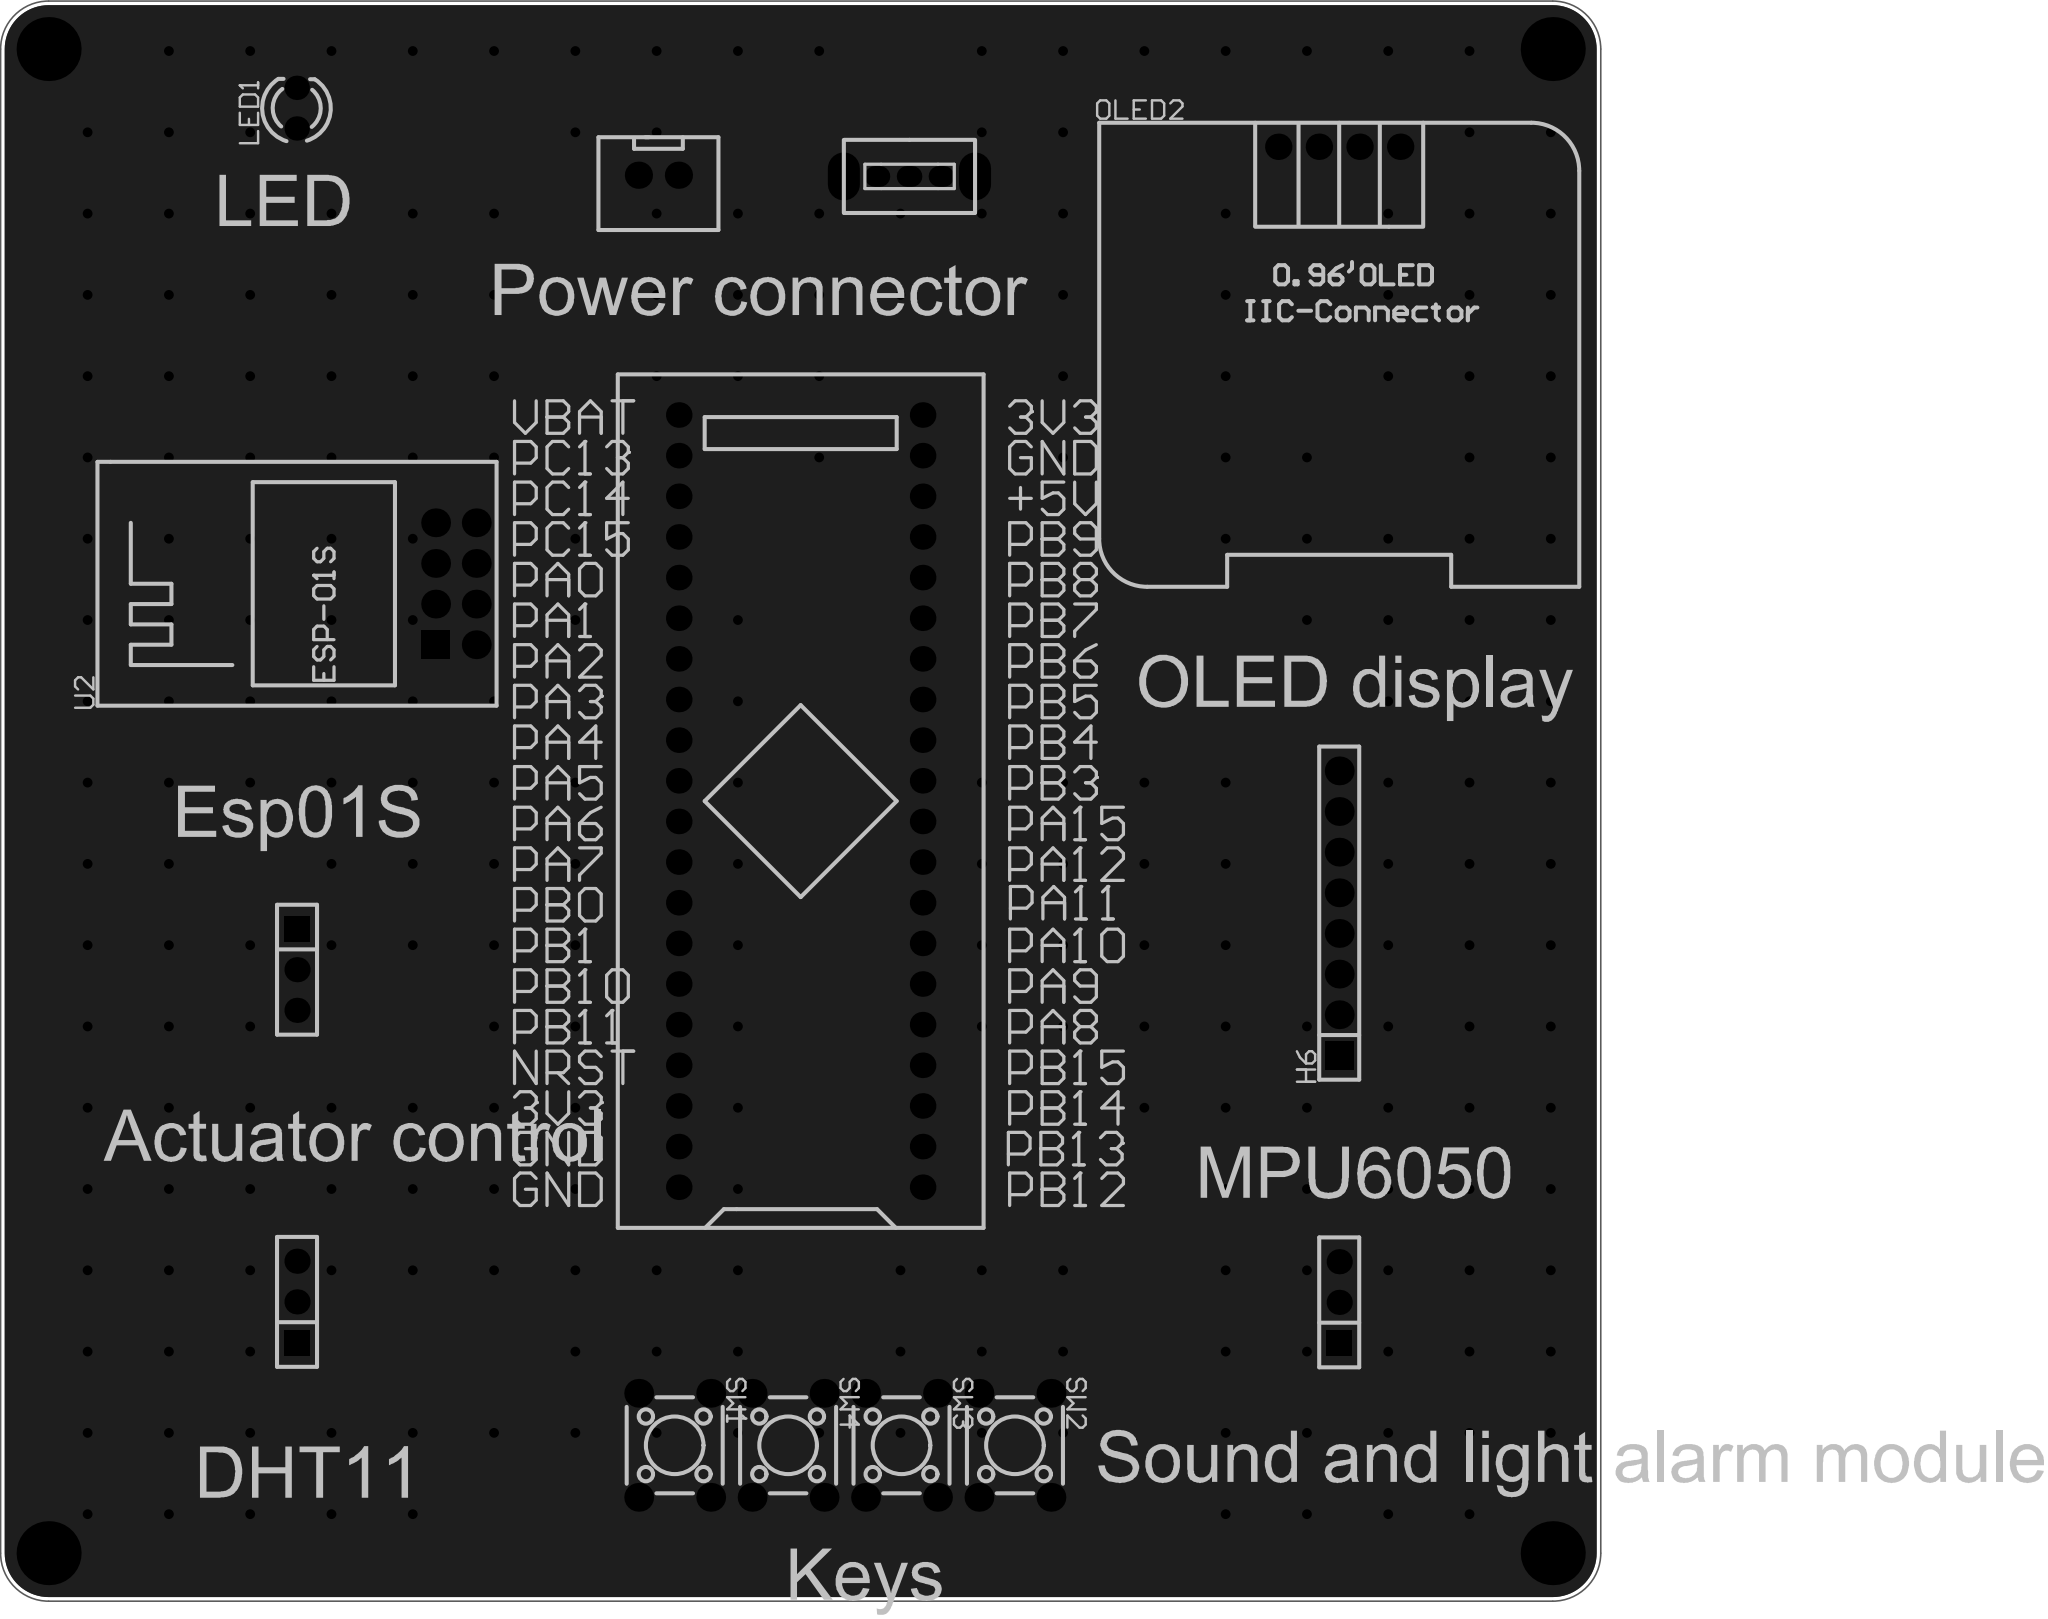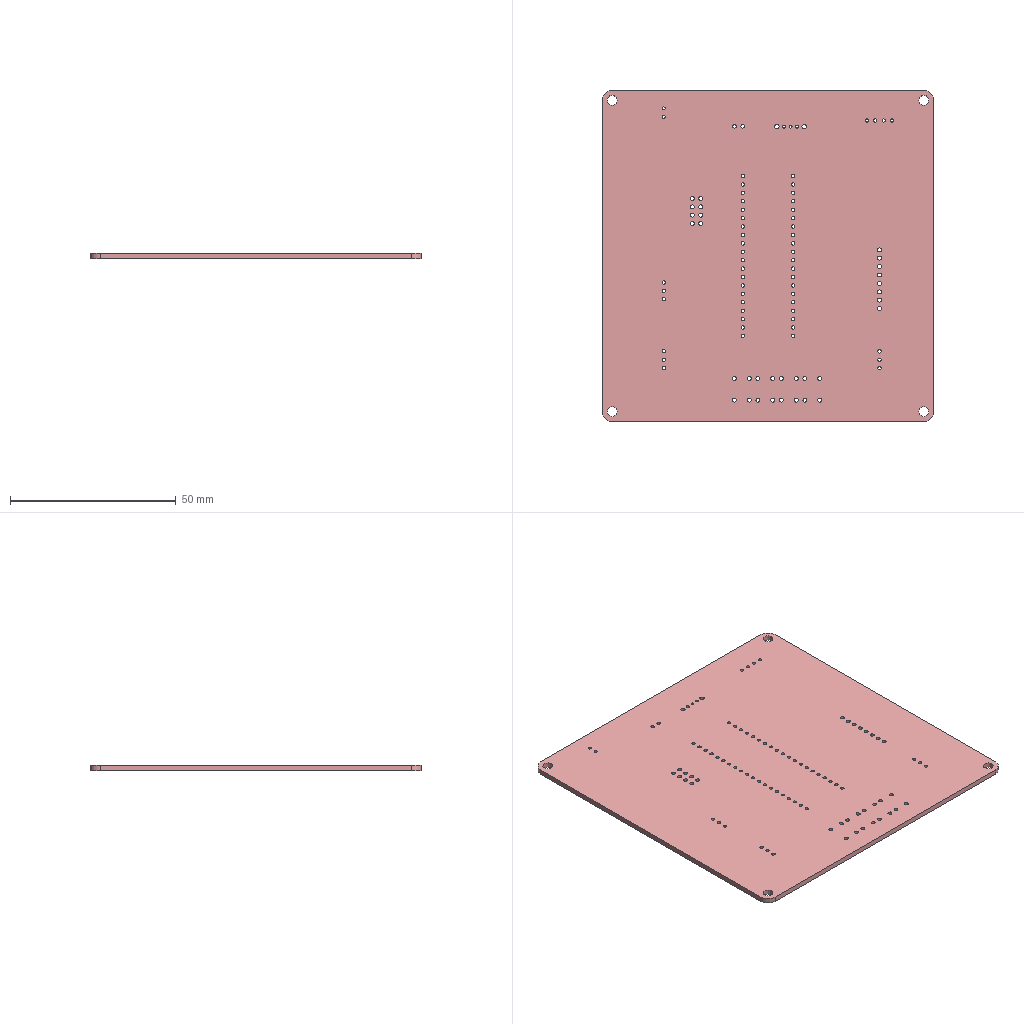Circuit board layout | Altium Designer | box 100 x 100 x 1.6 mm
Layer stack:
# Altium Designer layer stack of  (unit mm; dielectric type: 0 none, 1 core, 2 prepreg, 3 surface material)
index,name,kind,layer,copper_thickness_mm,dielectric_type,dielectric_thickness_mm,dielectric_material,dielectric_constant
0,Top Paste Mask Layer,other,,,,,,
1,Top Silkscreen Layer,other,,,,,,
2,Top Solder Mask Layer,dielectric,,,3,0.01,,3.3
3,Top Layer,copper,Top Layer,0.035,,,,
4,Dielectric1,dielectric,,,3,1.51,FR4,4.5
5,Bottom Layer,copper,Bottom Layer,0.035,,,,
6,Bottom Solder Mask Layer,dielectric,,,3,0.01,,3.3
7,Bottom Silkscreen Layer,other,,,,,,
8,Bottom Paste Mask Layer,other,,,,,,
# drill layer pairs: low layer,high layer
drill_pair,Top Layer,Bottom Layer
Part placement:
Designator,Comment,Layer,Footprint,Center-X(mm),Center-Y(mm),Rotation
U1,STM32F103C8T6-Card,TopLayer,CONN-TH_L53.3-W22.9_STM32F103C8T6-CARD,142.494,130.175,90
SW1,,TopLayer,SW-TH_4P-L6.0-W6.0-P4.50-LS6.5,134.62,89.916,270
SW2,,TopLayer,SW-TH_4P-L6.0-W6.0-P4.50-LS6.5,155.883,89.916,270
SW3,,TopLayer,SW-TH_4P-L6.0-W6.0-P4.50-LS6.5,148.796,89.916,270
SW4,,TopLayer,SW-TH_4P-L6.0-W6.0-P4.50-LS6.5,141.708,89.916,270
H12,,TopLayer,HDR-TH_3P-P2.54-V-F,111.018,119.639,270
CN4,XH2.54*2P_THT,TopLayer,CONN-TH_2P-P2.50-XH2.54-2P,133.604,169.291,0
SW5,,TopLayer,拨动开关,149.291,169.216,180
H1,,TopLayer,HDR-TH_3P-P2.54-V-F,176.149,98.849,90
H3,,TopLayer,HDR-TH_3P-P2.54-V-F,111.018,98.88,90
H6,,TopLayer,HDR-TH_8P-P2.54-V-F-1,176.149,123.175,90
OLED2,,TopLayer,0.96OLED_4P,176.149,171.069,0
U2,ESP-01S,TopLayer,WIFIM-TH_ESP-01S,120.949,143.759,90
LED1,,TopLayer,LED_TH-3mm,110.998,173.482,90
Pad and via stacks:
# Altium Designer via and pad stacks of  (unit mm). Each distinct definition once, with the count of objects using it.
# via: kind,start_layer,end_layer,hole_mm,diameter_mm,mode(0 simple;1 top-mid-bottom;2 full stack),diameter_per_layer,count,example_net
# pad: kind,layer,hole_mm,hole_type(0 round;1 square;2 slot),plating,top_size,top_shape(1 round;2 rect;3 octagon;9 rounded rect),mid_size,bottom_size,mode,footprint,size_per_layer,count,example
pad,Multi-Layer,3,0,plated,4x4,1,4x4,4x4,0,,,4,1
pad,Multi-Layer,1,0,plated,1.6x1.6,1,1.6x1.6,1.6x1.6,0,CONN-TH_L53.3-W22.9_STM32F103C8T6-CARD,,40,U1.1
pad,Multi-Layer,1.2,0,plated,1.8x1.8,1,1.8x1.8,1.8x1.8,0,SW-TH_4P-L6.0-W6.0-P4.50-LS6.5,,16,SW1.1
pad,Multi-Layer,1.02,0,plated,1.575x1.575,1,1.575x1.575,1.575x1.575,0,HDR-TH_3P-P2.54-V-F,,6,H12.3
pad,Multi-Layer,1.02,0,plated,1.575x1.575,2,1.575x1.575,1.575x1.575,0,HDR-TH_3P-P2.54-V-F,,3,H12.1
pad,Multi-Layer,1.05,0,plated,1.7x1.7,1,1.7x1.7,1.7x1.7,0,CONN-TH_2P-P2.50-XH2.54-2P,,2,CN4.2
pad,Multi-Layer,0.8992,0,plated,1.6x1.3,1,1.6x1.3,1.6x1.3,0,\u00B2\u00A6\u00B6\u00AF\u00BF\u00AA\u00B9\u00D8,,3,SW5.1
pad,Multi-Layer,1.3,0,plated,3x1.999,1,3x1.999,3x1.999,0,\u00B2\u00A6\u00B6\u00AF\u00BF\u00AA\u00B9\u00D8,,2,SW5.4
pad,Multi-Layer,1.2,0,plated,1.8x1.8,2,1.8x1.8,1.8x1.8,0,HDR-TH_8P-P2.54-V-F-1,,1,H6.1
pad,Multi-Layer,1.2,0,plated,1.8x1.8,1,1.8x1.8,1.8x1.8,0,HDR-TH_8P-P2.54-V-F-1,,7,H6.2
pad,Multi-Layer,1,0,plated,1.65x1.65,1,1.65x1.65,1.65x1.65,0,0.96OLED_4P,,4,OLED2.4
pad,Multi-Layer,1.2,0,plated,1.8x1.8,2,1.8x1.8,1.8x1.8,0,WIFIM-TH_ESP-01S,,1,U2.1
pad,Multi-Layer,1.2,0,plated,1.8x1.8,1,1.8x1.8,1.8x1.8,0,WIFIM-TH_ESP-01S,,7,U2.2
pad,Multi-Layer,0.9144,0,plated,1.524x1.524,1,1.524x1.524,1.524x1.524,0,LED_TH-3mm,,2,LED1.1
via,Top Layer,Bottom Layer,0.3048,0.61,0,,257,GND
Copper pours:
name,layer,net,type(0 solid;1 hatched;2 none)
Bottom Layer-GND,Bottom Layer,GND,0
Top Layer-GND,Top Layer,GND,0
Design rules, without the lines most boards share:
# Altium Designer design rules of  (exported by Altium Designer, unit mm)
# columns: name | kind | enabled | priority | scope1 | scope2 | descriptor | typed fields (field=value)
Copper_copperRegion_copperThickness1oz | 0 | disabled | 4 | All | All | Clearance Constraint (Gap=5.984mil) (Disabled)(All),(All) | gap=0.152
Copper_copperRegion_copperThickness1oz_1 | 63 | disabled | 4 | All | All | Board Clearance Constraint (Gap=0mil) (Disabled)(All) |
Copper_copperRegion_Copper_copperRegion | 0 | disabled | 5 | All | All | Clearance Constraint (Gap=5.984mil) (Disabled)(All),(All) | gap=0.152
Copper_copperRegion_Copper_copperRegion_1 | 63 | disabled | 5 | All | All | Board Clearance Constraint (Gap=0mil) (Disabled)(All) |
copperThickness1oz | 0 | enabled | 6 | All | All | Clearance Constraint (Gap=5.984mil) (All),(All) | gap=0.152
copperThickness1oz_1 | 63 | enabled | 6 | All | All | Board Clearance Constraint (Gap=0mil) (All) |
copperRegion_copperThickness1oz | 20 | disabled | 1 | All | All | Polygon Connect Rule(Relief Connect )(Conductor Width=10mil) (Relief Angle=90 Angle) (Entries=4) (Air Gap Width=10mil) (Disabled)(All),(All) | connect_style(0=relief,1=direct,2=none)=0 relief_conductor_width=0.254 relief_entries=4
copperRegion_Copper_copperRegion | 20 | disabled | 2 | All | All | Polygon Connect Rule(Relief Connect )(Conductor Width=10mil) (Relief Angle=90 Angle) (Entries=4) (Air Gap Width=10mil) (Disabled)(All),(All) | connect_style(0=relief,1=direct,2=none)=0 relief_conductor_width=0.254 relief_entries=4
copperRegion | 20 | enabled | 3 | All | All | Polygon Connect Rule(Relief Connect )(Conductor Width=10mil) (Relief Angle=90 Angle) (Entries=4) (Air Gap Width=10mil) (All),(All) | connect_style(0=relief,1=direct,2=none)=0 relief_conductor_width=0.254 relief_entries=4